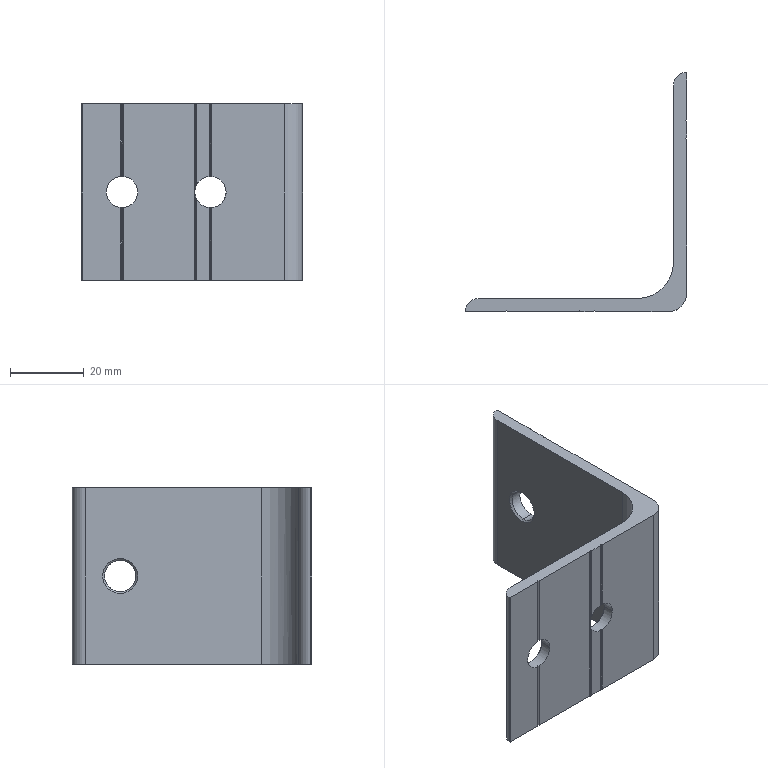Part | STEP file | 31E-01020QY13 | 1 solid | 65 faces | box 60 x 64.996 x 48 mm | volume 20307 mm3 | cylinder 30 | plane 29 | cone 6 | commonest cylinder face diameters 0.2 x17 8.5 x6 0.4 x3 7 x2 10 x1 20 x1